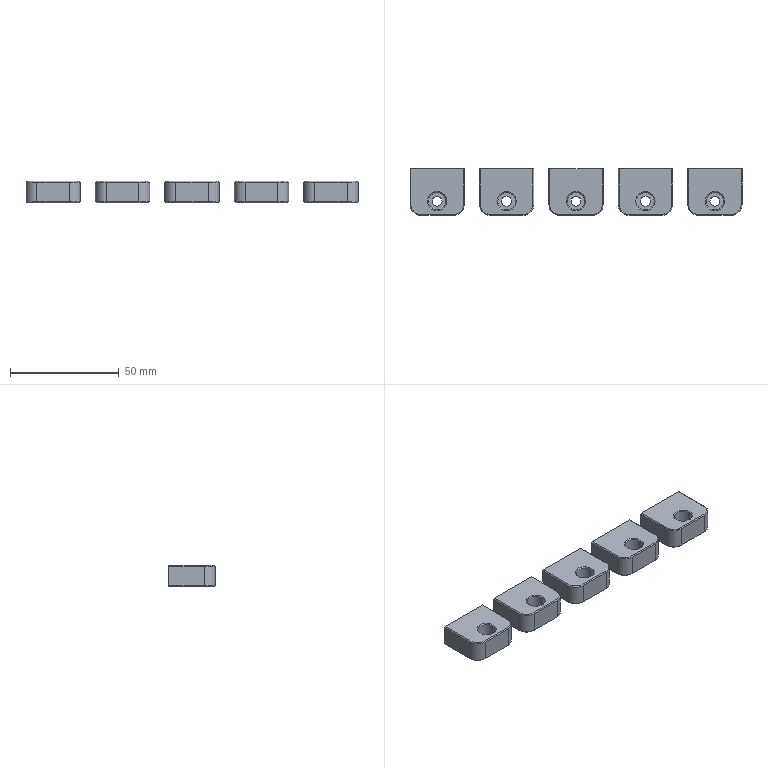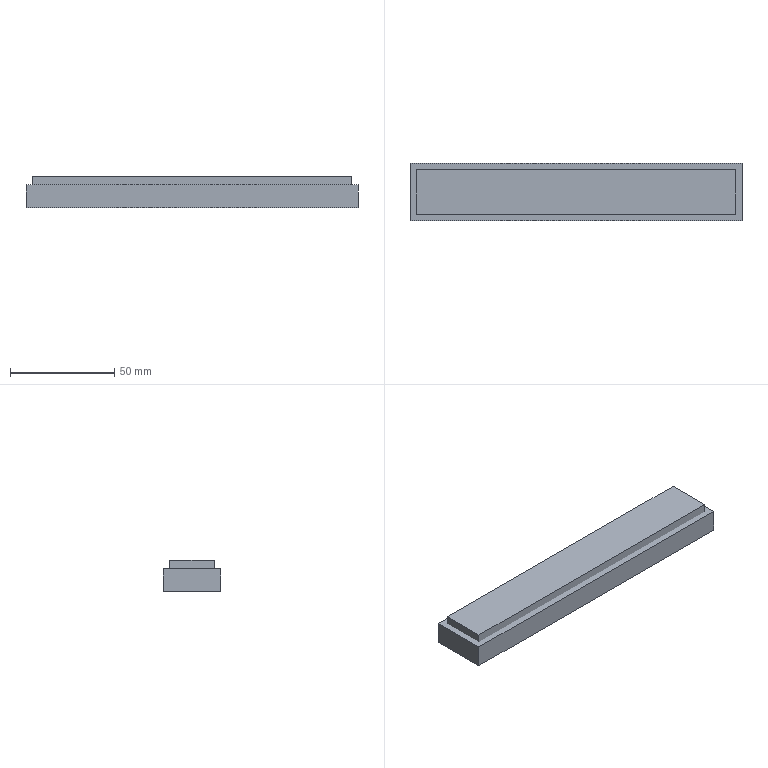CAM job | NX | 3+2 milling, drilling | part box 153 x 21.5 x 10 mm | stock box 159 x 27.5 x 15 mm
Tools:
number,name,description,diameter,corner_radius,flute_length,length,flutes
2,D4A45,Milling Tool-5 Parameters,4.0,0.0,2.0,2.0,2
1,D63,Milling Tool-5 Parameters,63.0,0.0,50.0,75.0,2
14,4.5ZT,Drilling Tool,4.5,0.0,35.0,50.0,2
6,D6,Milling Tool-5 Parameters,6.0,0.0,50.0,75.0,2
15,3.5ZT,Drilling Tool,3.5,0.0,35.0,50.0,2
Operations:
program,operation,operation_type,tool,method,geometry_group,spindle_rpm,surface_speed,feed_per_tooth,feed_cut,feed_plunge,cut_length_mm,path_length_mm,cut_time_min,machine_time_min
1虎钳,FLOOR_WALL,VolumeBased25DMillingOperation,D63,METHOD,A,6500.0,1286.0,0.0962,1250.0,100.0,234.0,288.0,0.1872,0.1926
1虎钳,DRILLING_COPY,Operation,D4A45,METHOD,A,5000.0,62.0,0.025,250.0,0.0,20.0,240.561,0.08,0.1021
1虎钳,DRILLING_COPY_COPY_COPY_COPY_COPY,Operation,4.5ZT,METHOD,A,1910.0,21.0,0.0471,180.0,0.0,79.26,359.081,0.4403,0.4683
1虎钳,ZLEVEL_PROFILE_1_COPY_1_COPY_COPY,ZLevelMilling,D4A45,METHOD,A,9500.0,179.0,0.0526,1000.0,100.0,615.104,1495.342,0.6151,0.7031
1虎钳,HOLE_MILLING,CylinderMilling,D6,METHOD,A,9500.0,179.0,0.0789,1500.0,100.0,612.911,1070.911,0.4086,0.4544
1虎钳,ZLEVEL_PROFILE_COPY_COPY_1_COPY,ZLevelMilling,D6,METHOD,A,9500.0,179.0,0.1158,2200.0,1000.0,11160.61,11682.45,5.177,5.229
1虎钳,ZLEVEL_PROFILE_COPY_COPY_COPY_COPY,ZLevelMilling,D6,MILL_FINISH,A,9500.0,119.0,0.0632,1200.0,1000.0,562.2,1299.2,0.4705,0.5442
2,DRILLING_COPY_COPY,Operation,D4A45,METHOD,B,5000.0,62.0,0.025,250.0,0.0,48.5,325.016,0.194,0.2217
2,DRILLING_COPY_COPY_COPY_COPY_COPY_COPY_1,Operation,3.5ZT,METHOD,B,1910.0,21.0,0.0471,180.0,0.0,130.515,489.046,0.7251,0.7609
3,FLOOR_WALL_COPY,VolumeBased25DMillingOperation,D63,METHOD,C,6500.0,1286.0,0.0962,1250.0,100.0,1140.0,2278.001,0.912,1.026
3,ZLEVEL_PROFILE_1_COPY_1_COPY_COPY_COPY,ZLevelMilling,D4A45,METHOD,C,9500.0,179.0,0.0526,1000.0,100.0,557.546,1431.655,0.5575,0.645